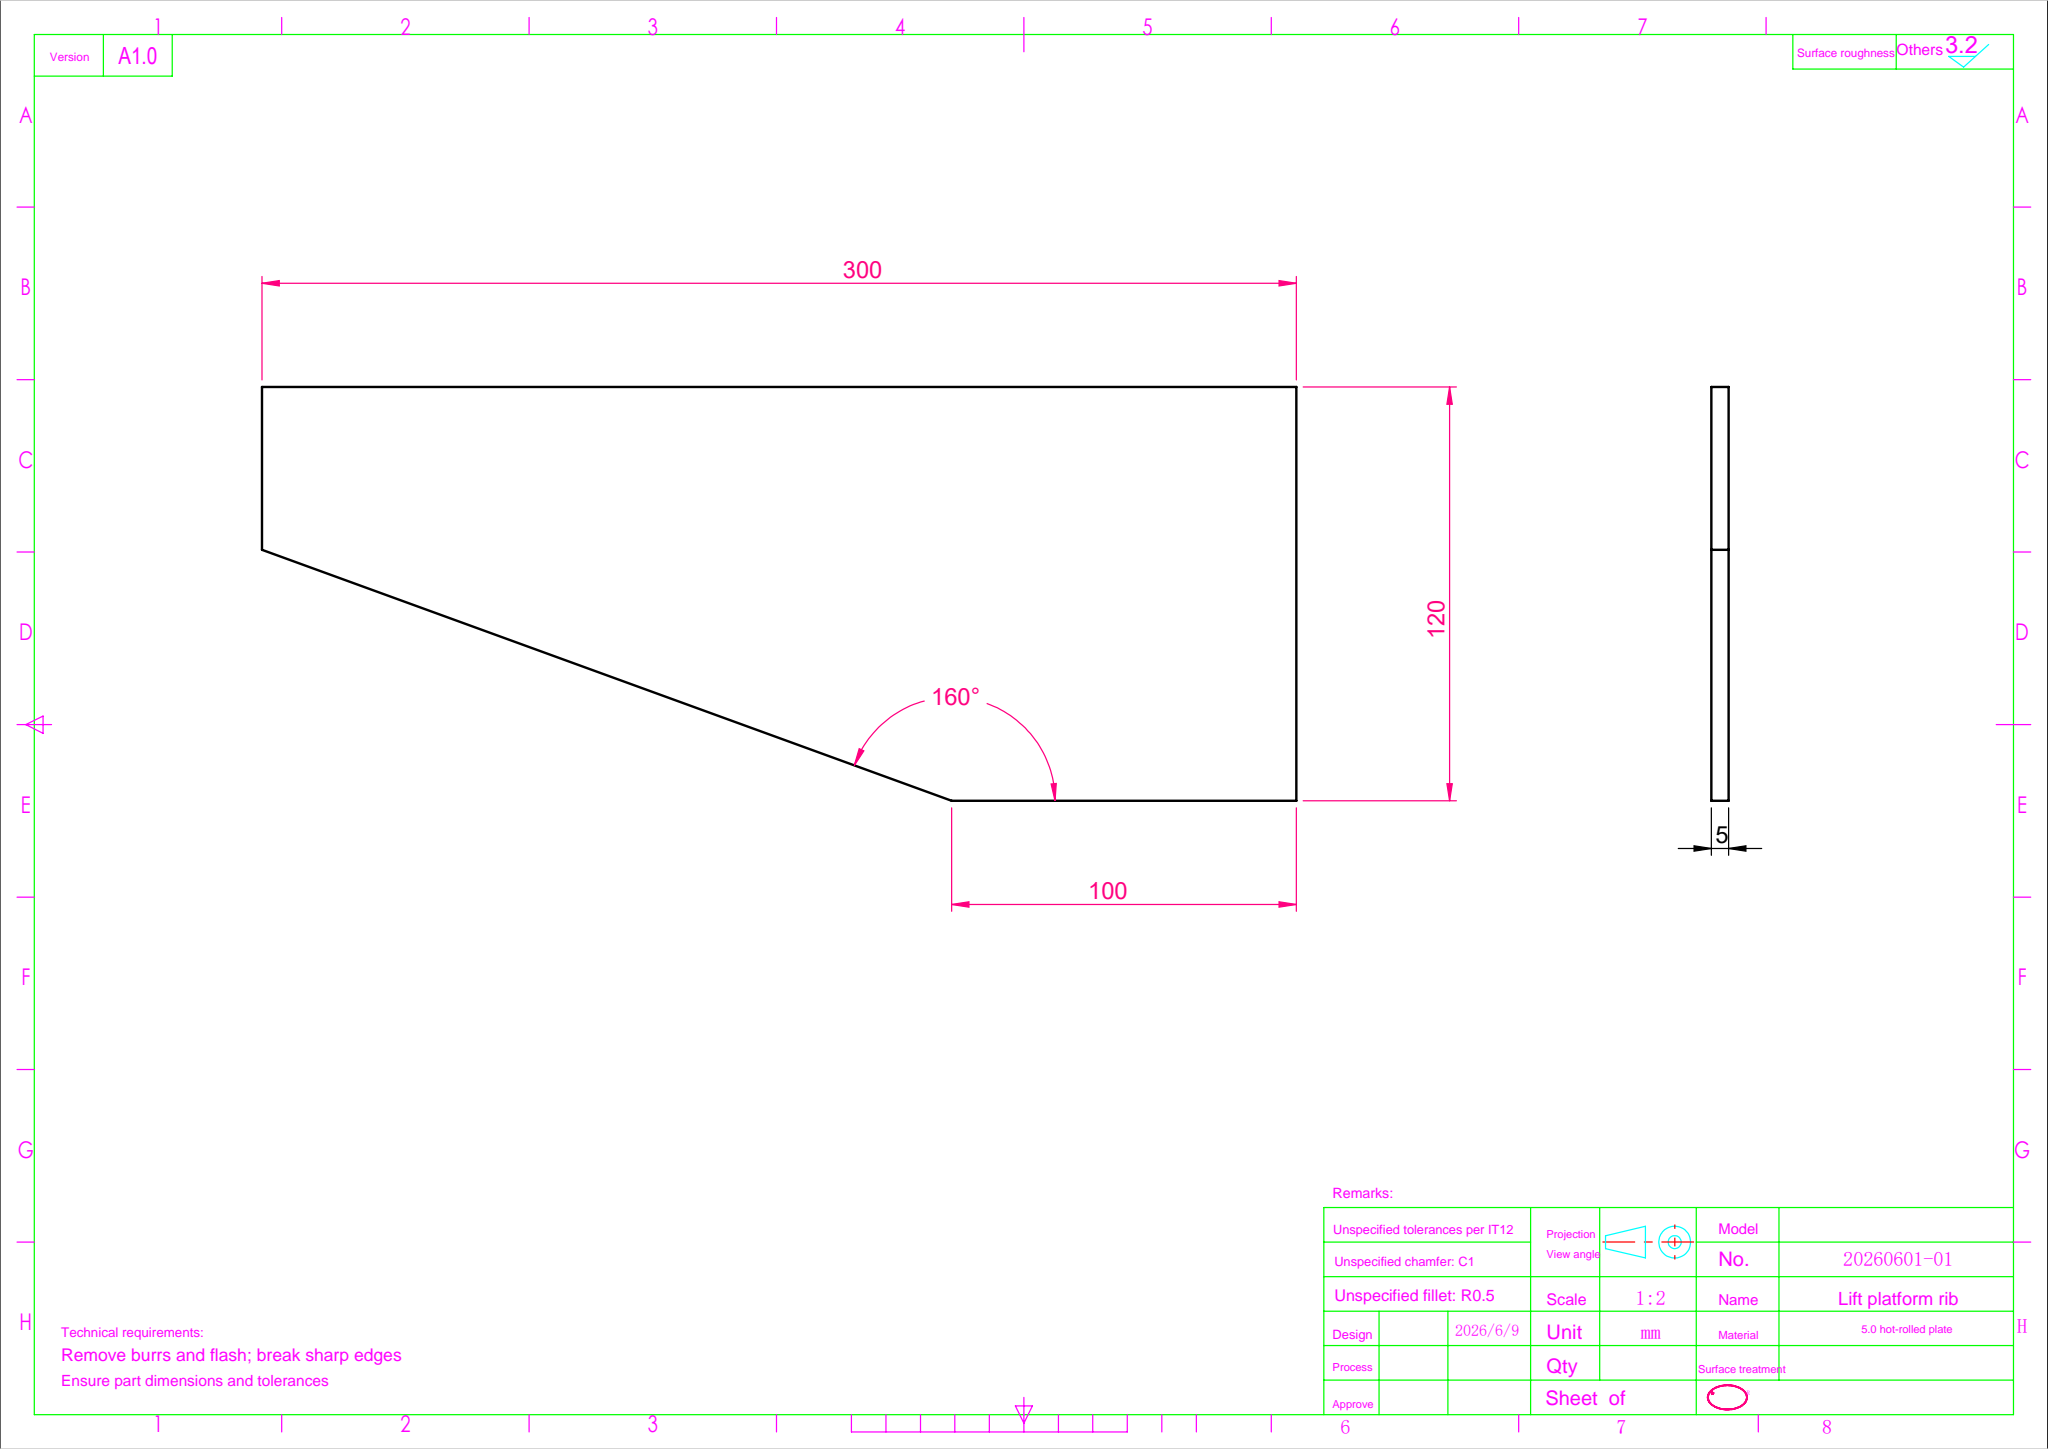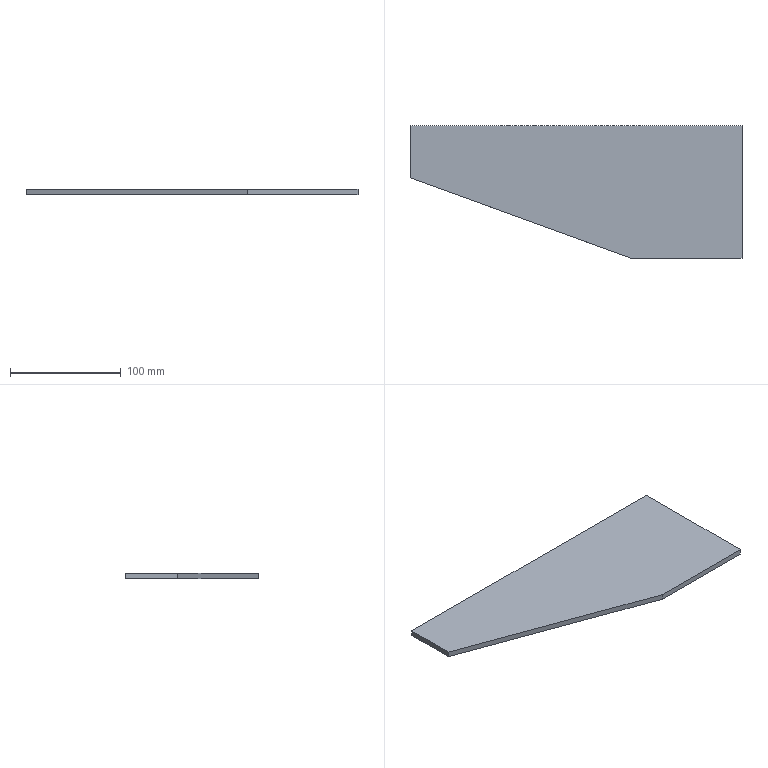Part | SolidWorks | features Extrusion 1 | 1 solid | 7 faces | box 300 x 120 x 5 mm | volume 143603 mm3 | plane 7
STEP:
#1=CARTESIAN_POINT('',(0.,0.,0.));
#2=VERTEX_POINT('',#1);
#3=CARTESIAN_POINT('',(0.,-47.206,0.));
#4=VERTEX_POINT('',#3);
#5=CARTESIAN_POINT('',(0.,-47.206,0.));
#6=DIRECTION('',(0.,-1.,0.));
#7=VECTOR('',#6,1000.);
#8=LINE('',#5,#7);
#9=EDGE_CURVE('',#2,#4,#8,.T.);
#10=ORIENTED_EDGE('',*,*,#9,.T.);
#11=CARTESIAN_POINT('',(0.,-47.206,5.));
#12=VERTEX_POINT('',#11);
#13=CARTESIAN_POINT('',(0.,-47.206,5.));
#14=DIRECTION('',(0.,0.,-1.));
#15=VECTOR('',#14,1000.);
#16=LINE('',#13,#15);
#17=EDGE_CURVE('',#12,#4,#16,.T.);
#18=ORIENTED_EDGE('',*,*,#17,.F.);
#19=CARTESIAN_POINT('',(0.,0.,5.));
#20=VERTEX_POINT('',#19);
#21=CARTESIAN_POINT('',(0.,-47.206,5.));
#22=DIRECTION('',(0.,-1.,0.));
#23=VECTOR('',#22,1000.);
#24=LINE('',#21,#23);
#25=EDGE_CURVE('',#20,#12,#24,.T.);
#26=ORIENTED_EDGE('',*,*,#25,.F.);
#27=CARTESIAN_POINT('',(0.,0.,5.));
#28=DIRECTION('',(0.,0.,-1.));
#29=VECTOR('',#28,1000.);
#30=LINE('',#27,#29);
#31=EDGE_CURVE('',#20,#2,#30,.T.);
#32=ORIENTED_EDGE('',*,*,#31,.T.);
#33=EDGE_LOOP('',(#10,#18,#26,#32));
#34=FACE_OUTER_BOUND('',#33,.T.);
#35=CARTESIAN_POINT('',(0.,-47.206,5.));
#36=DIRECTION('',(1.,0.,0.));
#37=DIRECTION('',(0.,1.,0.));
#38=AXIS2_PLACEMENT_3D('',#35,#36,#37);
#39=PLANE('',#38);
#40=ADVANCED_FACE('',(#34),#39,.F.);
#41=CARTESIAN_POINT('',(200.,-120.,0.));
#42=VERTEX_POINT('',#41);
#43=CARTESIAN_POINT('',(200.,-120.,0.));
#44=DIRECTION('',(0.9397,-0.342,0.));
#45=VECTOR('',#44,1000.);
#46=LINE('',#43,#45);
#47=EDGE_CURVE('',#4,#42,#46,.T.);
#48=ORIENTED_EDGE('',*,*,#47,.T.);
#49=CARTESIAN_POINT('',(200.,-120.,5.));
#50=VERTEX_POINT('',#49);
#51=CARTESIAN_POINT('',(200.,-120.,5.));
#52=DIRECTION('',(0.,0.,-1.));
#53=VECTOR('',#52,1000.);
#54=LINE('',#51,#53);
#55=EDGE_CURVE('',#50,#42,#54,.T.);
#56=ORIENTED_EDGE('',*,*,#55,.F.);
#57=CARTESIAN_POINT('',(200.,-120.,5.));
#58=DIRECTION('',(0.9397,-0.342,0.));
#59=VECTOR('',#58,1000.);
#60=LINE('',#57,#59);
#61=EDGE_CURVE('',#12,#50,#60,.T.);
#62=ORIENTED_EDGE('',*,*,#61,.F.);
#63=ORIENTED_EDGE('',*,*,#17,.T.);
#64=EDGE_LOOP('',(#48,#56,#62,#63));
#65=FACE_OUTER_BOUND('',#64,.T.);
#66=CARTESIAN_POINT('',(200.,-120.,5.));
#67=DIRECTION('',(0.342,0.9397,0.));
#68=DIRECTION('',(-0.9397,0.342,0.));
#69=AXIS2_PLACEMENT_3D('',#66,#67,#68);
#70=PLANE('',#69);
#71=ADVANCED_FACE('',(#65),#70,.F.);
#72=CARTESIAN_POINT('',(300.,-120.,0.));
#73=VERTEX_POINT('',#72);
#74=CARTESIAN_POINT('',(300.,-120.,0.));
#75=DIRECTION('',(1.,0.,0.));
#76=VECTOR('',#75,1000.);
#77=LINE('',#74,#76);
#78=EDGE_CURVE('',#42,#73,#77,.T.);
#79=ORIENTED_EDGE('',*,*,#78,.T.);
#80=CARTESIAN_POINT('',(300.,-120.,5.));
#81=VERTEX_POINT('',#80);
#82=CARTESIAN_POINT('',(300.,-120.,5.));
#83=DIRECTION('',(0.,0.,-1.));
#84=VECTOR('',#83,1000.);
#85=LINE('',#82,#84);
#86=EDGE_CURVE('',#81,#73,#85,.T.);
#87=ORIENTED_EDGE('',*,*,#86,.F.);
#88=CARTESIAN_POINT('',(300.,-120.,5.));
#89=DIRECTION('',(1.,0.,0.));
#90=VECTOR('',#89,1000.);
#91=LINE('',#88,#90);
#92=EDGE_CURVE('',#50,#81,#91,.T.);
#93=ORIENTED_EDGE('',*,*,#92,.F.);
#94=ORIENTED_EDGE('',*,*,#55,.T.);
#95=EDGE_LOOP('',(#79,#87,#93,#94));
#96=FACE_OUTER_BOUND('',#95,.T.);
#97=CARTESIAN_POINT('',(300.,-120.,5.));
#98=DIRECTION('',(0.,1.,0.));
#99=DIRECTION('',(-1.,0.,0.));
#100=AXIS2_PLACEMENT_3D('',#97,#98,#99);
#101=PLANE('',#100);
#102=ADVANCED_FACE('',(#96),#101,.F.);
#103=CARTESIAN_POINT('',(300.,0.,0.));
#104=VERTEX_POINT('',#103);
#105=CARTESIAN_POINT('',(300.,0.,0.));
#106=DIRECTION('',(0.,1.,0.));
#107=VECTOR('',#106,1000.);
#108=LINE('',#105,#107);
#109=EDGE_CURVE('',#73,#104,#108,.T.);
#110=ORIENTED_EDGE('',*,*,#109,.T.);
#111=CARTESIAN_POINT('',(300.,0.,5.));
#112=VERTEX_POINT('',#111);
#113=CARTESIAN_POINT('',(300.,0.,5.));
#114=DIRECTION('',(0.,0.,-1.));
#115=VECTOR('',#114,1000.);
#116=LINE('',#113,#115);
#117=EDGE_CURVE('',#112,#104,#116,.T.);
#118=ORIENTED_EDGE('',*,*,#117,.F.);
#119=CARTESIAN_POINT('',(300.,0.,5.));
#120=DIRECTION('',(0.,1.,0.));
#121=VECTOR('',#120,1000.);
#122=LINE('',#119,#121);
#123=EDGE_CURVE('',#81,#112,#122,.T.);
#124=ORIENTED_EDGE('',*,*,#123,.F.);
#125=ORIENTED_EDGE('',*,*,#86,.T.);
#126=EDGE_LOOP('',(#110,#118,#124,#125));
#127=FACE_OUTER_BOUND('',#126,.T.);
#128=CARTESIAN_POINT('',(300.,0.,5.));
#129=DIRECTION('',(-1.,0.,0.));
#130=DIRECTION('',(0.,0.,1.));
#131=AXIS2_PLACEMENT_3D('',#128,#129,#130);
#132=PLANE('',#131);
#133=ADVANCED_FACE('',(#127),#132,.F.);
#134=CARTESIAN_POINT('',(0.,0.,0.));
#135=DIRECTION('',(-1.,0.,0.));
#136=VECTOR('',#135,1000.);
#137=LINE('',#134,#136);
#138=EDGE_CURVE('',#104,#2,#137,.T.);
#139=ORIENTED_EDGE('',*,*,#138,.T.);
#140=ORIENTED_EDGE('',*,*,#31,.F.);
#141=CARTESIAN_POINT('',(0.,0.,5.));
#142=DIRECTION('',(-1.,0.,0.));
#143=VECTOR('',#142,1000.);
#144=LINE('',#141,#143);
#145=EDGE_CURVE('',#112,#20,#144,.T.);
#146=ORIENTED_EDGE('',*,*,#145,.F.);
#147=ORIENTED_EDGE('',*,*,#117,.T.);
#148=EDGE_LOOP('',(#139,#140,#146,#147));
#149=FACE_OUTER_BOUND('',#148,.T.);
#150=CARTESIAN_POINT('',(0.,0.,5.));
#151=DIRECTION('',(0.,-1.,0.));
#152=DIRECTION('',(0.,0.,-1.));
#153=AXIS2_PLACEMENT_3D('',#150,#151,#152);
#154=PLANE('',#153);
#155=ADVANCED_FACE('',(#149),#154,.F.);
#156=ORIENTED_EDGE('',*,*,#25,.T.);
#157=ORIENTED_EDGE('',*,*,#61,.T.);
#158=ORIENTED_EDGE('',*,*,#92,.T.);
#159=ORIENTED_EDGE('',*,*,#123,.T.);
#160=ORIENTED_EDGE('',*,*,#145,.T.);
#161=EDGE_LOOP('',(#156,#157,#158,#159,#160));
#162=FACE_OUTER_BOUND('',#161,.T.);
#163=CARTESIAN_POINT('',(0.,0.,5.));
#164=DIRECTION('',(0.,0.,-1.));
#165=DIRECTION('',(-1.,0.,0.));
#166=AXIS2_PLACEMENT_3D('',#163,#164,#165);
#167=PLANE('',#166);
#168=ADVANCED_FACE('',(#162),#167,.F.);
#169=ORIENTED_EDGE('',*,*,#9,.F.);
#170=ORIENTED_EDGE('',*,*,#138,.F.);
#171=ORIENTED_EDGE('',*,*,#109,.F.);
#172=ORIENTED_EDGE('',*,*,#78,.F.);
#173=ORIENTED_EDGE('',*,*,#47,.F.);
#174=EDGE_LOOP('',(#169,#170,#171,#172,#173));
#175=FACE_OUTER_BOUND('',#174,.T.);
#176=CARTESIAN_POINT('',(0.,0.,0.));
#177=DIRECTION('',(0.,0.,-1.));
#178=DIRECTION('',(-1.,0.,0.));
#179=AXIS2_PLACEMENT_3D('',#176,#177,#178);
#180=PLANE('',#179);
#181=ADVANCED_FACE('',(#175),#180,.T.);
#182=CLOSED_SHELL('',(#40,#71,#102,#133,#155,#168,#181));
#183=MANIFOLD_SOLID_BREP('',#182);
#184=CARTESIAN_POINT('',(0.,0.,0.));
#185=DIRECTION('',(0.,0.,1.));
#186=DIRECTION('',(1.,0.,0.));
#187=AXIS2_PLACEMENT_3D('',#184,#185,#186);
#188=(LENGTH_UNIT()NAMED_UNIT(*)SI_UNIT(.MILLI.,.METRE.));
#189=UNCERTAINTY_MEASURE_WITH_UNIT(LENGTH_MEASURE(0.00001),#188,'','');
#190=(NAMED_UNIT(*)PLANE_ANGLE_UNIT()SI_UNIT($,.RADIAN.));
#191=(NAMED_UNIT(*)SI_UNIT($,.STERADIAN.)SOLID_ANGLE_UNIT());
#192=(GEOMETRIC_REPRESENTATION_CONTEXT(3)GLOBAL_UNCERTAINTY_ASSIGNED_CONTEXT((#189))GLOBAL_UNIT_ASSIGNED_CONTEXT((#188,#190,#191))REPRESENTATION_CONTEXT('',''));
#193=ADVANCED_BREP_SHAPE_REPRESENTATION('',(#183,#187),#192);